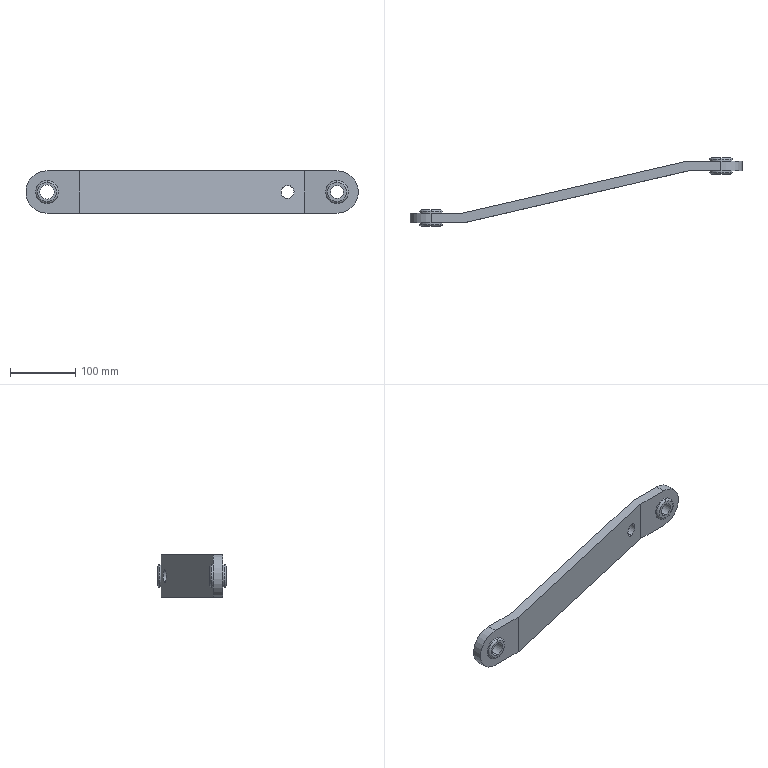Part | SolidWorks | 1 solid | 36 faces | box 510.518 x 105 x 65 mm | volume 489274 mm3 | cylinder 16 | plane 12 | torus 8 | commonest cylinder face diameters 35 x8 20 x4 22 x2 65 x2
STEP:
#1=CARTESIAN_POINT('',(396.018,97.,-17.5));
#2=VERTEX_POINT('',#1);
#3=CARTESIAN_POINT('',(396.018,97.,17.5));
#4=VERTEX_POINT('',#3);
#5=CARTESIAN_POINT('',(396.018,97.,0.));
#6=DIRECTION('',(0.,-1.,0.));
#7=DIRECTION('',(0.,0.,1.));
#8=AXIS2_PLACEMENT_3D('',#5,#6,#7);
#9=CIRCLE('',#8,17.5);
#10=EDGE_CURVE('',#2,#4,#9,.T.);
#11=ORIENTED_EDGE('',*,*,#10,.F.);
#12=CARTESIAN_POINT('',(396.018,100.,-14.5));
#13=VERTEX_POINT('',#12);
#14=CARTESIAN_POINT('',(396.018,97.,-14.5));
#15=DIRECTION('',(1.,0.,0.));
#16=DIRECTION('',(0.,0.,-1.));
#17=AXIS2_PLACEMENT_3D('',#14,#15,#16);
#18=CIRCLE('',#17,3.);
#19=EDGE_CURVE('',#2,#13,#18,.T.);
#20=ORIENTED_EDGE('',*,*,#19,.T.);
#21=CARTESIAN_POINT('',(396.018,100.,14.5));
#22=VERTEX_POINT('',#21);
#23=CARTESIAN_POINT('',(396.018,100.,0.));
#24=DIRECTION('',(0.,1.,0.));
#25=DIRECTION('',(0.,0.,1.));
#26=AXIS2_PLACEMENT_3D('',#23,#24,#25);
#27=CIRCLE('',#26,14.5);
#28=EDGE_CURVE('',#22,#13,#27,.T.);
#29=ORIENTED_EDGE('',*,*,#28,.F.);
#30=CARTESIAN_POINT('',(396.018,97.,14.5));
#31=DIRECTION('',(-1.,0.,0.));
#32=DIRECTION('',(0.,0.,1.));
#33=AXIS2_PLACEMENT_3D('',#30,#31,#32);
#34=CIRCLE('',#33,3.);
#35=EDGE_CURVE('',#4,#22,#34,.T.);
#36=ORIENTED_EDGE('',*,*,#35,.F.);
#37=EDGE_LOOP('',(#11,#20,#29,#36));
#38=FACE_OUTER_BOUND('',#37,.T.);
#39=CARTESIAN_POINT('',(396.018,97.,0.));
#40=DIRECTION('',(0.,1.,0.));
#41=DIRECTION('',(0.,0.,1.));
#42=AXIS2_PLACEMENT_3D('',#39,#40,#41);
#43=TOROIDAL_SURFACE('',#42,14.5,3.);
#44=ADVANCED_FACE('',(#38),#43,.T.);
#45=CARTESIAN_POINT('',(396.018,75.,-14.5));
#46=VERTEX_POINT('',#45);
#47=CARTESIAN_POINT('',(396.018,75.,14.5));
#48=VERTEX_POINT('',#47);
#49=CARTESIAN_POINT('',(396.018,75.,0.));
#50=DIRECTION('',(0.,-1.,0.));
#51=DIRECTION('',(0.,0.,1.));
#52=AXIS2_PLACEMENT_3D('',#49,#50,#51);
#53=CIRCLE('',#52,14.5);
#54=EDGE_CURVE('',#46,#48,#53,.T.);
#55=ORIENTED_EDGE('',*,*,#54,.F.);
#56=CARTESIAN_POINT('',(396.018,78.,-17.5));
#57=VERTEX_POINT('',#56);
#58=CARTESIAN_POINT('',(396.018,78.,-14.5));
#59=DIRECTION('',(1.,0.,0.));
#60=DIRECTION('',(0.,0.,-1.));
#61=AXIS2_PLACEMENT_3D('',#58,#59,#60);
#62=CIRCLE('',#61,3.);
#63=EDGE_CURVE('',#46,#57,#62,.T.);
#64=ORIENTED_EDGE('',*,*,#63,.T.);
#65=CARTESIAN_POINT('',(396.018,78.,17.5));
#66=VERTEX_POINT('',#65);
#67=CARTESIAN_POINT('',(396.018,78.,0.));
#68=DIRECTION('',(0.,1.,0.));
#69=DIRECTION('',(0.,0.,1.));
#70=AXIS2_PLACEMENT_3D('',#67,#68,#69);
#71=CIRCLE('',#70,17.5);
#72=EDGE_CURVE('',#66,#57,#71,.T.);
#73=ORIENTED_EDGE('',*,*,#72,.F.);
#74=CARTESIAN_POINT('',(396.018,78.,14.5));
#75=DIRECTION('',(-1.,0.,0.));
#76=DIRECTION('',(0.,0.,1.));
#77=AXIS2_PLACEMENT_3D('',#74,#75,#76);
#78=CIRCLE('',#77,3.);
#79=EDGE_CURVE('',#48,#66,#78,.T.);
#80=ORIENTED_EDGE('',*,*,#79,.F.);
#81=EDGE_LOOP('',(#55,#64,#73,#80));
#82=FACE_OUTER_BOUND('',#81,.T.);
#83=CARTESIAN_POINT('',(396.018,78.,0.));
#84=DIRECTION('',(0.,1.,0.));
#85=DIRECTION('',(0.,0.,1.));
#86=AXIS2_PLACEMENT_3D('',#83,#84,#85);
#87=TOROIDAL_SURFACE('',#86,14.5,3.);
#88=ADVANCED_FACE('',(#82),#87,.T.);
#89=ORIENTED_EDGE('',*,*,#72,.T.);
#90=CARTESIAN_POINT('',(396.018,80.,-17.5));
#91=VERTEX_POINT('',#90);
#92=CARTESIAN_POINT('',(396.018,75.,-17.5));
#93=DIRECTION('',(0.,1.,0.));
#94=VECTOR('',#93,1000.);
#95=LINE('',#92,#94);
#96=EDGE_CURVE('',#57,#91,#95,.T.);
#97=ORIENTED_EDGE('',*,*,#96,.T.);
#98=CARTESIAN_POINT('',(396.018,80.,17.5));
#99=VERTEX_POINT('',#98);
#100=CARTESIAN_POINT('',(396.018,80.,0.));
#101=DIRECTION('',(0.,-1.,0.));
#102=DIRECTION('',(0.,0.,-1.));
#103=AXIS2_PLACEMENT_3D('',#100,#101,#102);
#104=CIRCLE('',#103,17.5);
#105=EDGE_CURVE('',#91,#99,#104,.T.);
#106=ORIENTED_EDGE('',*,*,#105,.T.);
#107=CARTESIAN_POINT('',(396.018,75.,17.5));
#108=DIRECTION('',(0.,1.,0.));
#109=VECTOR('',#108,1000.);
#110=LINE('',#107,#109);
#111=EDGE_CURVE('',#66,#99,#110,.T.);
#112=ORIENTED_EDGE('',*,*,#111,.F.);
#113=EDGE_LOOP('',(#89,#97,#106,#112));
#114=FACE_OUTER_BOUND('',#113,.T.);
#115=CARTESIAN_POINT('',(396.018,75.,0.));
#116=DIRECTION('',(0.,1.,0.));
#117=DIRECTION('',(0.,0.,1.));
#118=AXIS2_PLACEMENT_3D('',#115,#116,#117);
#119=CYLINDRICAL_SURFACE('',#118,17.5);
#120=ADVANCED_FACE('',(#114),#119,.T.);
#121=CARTESIAN_POINT('',(396.018,75.,10.));
#122=VERTEX_POINT('',#121);
#123=CARTESIAN_POINT('',(396.018,75.,-10.));
#124=VERTEX_POINT('',#123);
#125=CARTESIAN_POINT('',(396.018,75.,0.));
#126=DIRECTION('',(0.,-1.,0.));
#127=DIRECTION('',(0.,0.,1.));
#128=AXIS2_PLACEMENT_3D('',#125,#126,#127);
#129=CIRCLE('',#128,10.);
#130=EDGE_CURVE('',#122,#124,#129,.T.);
#131=ORIENTED_EDGE('',*,*,#130,.T.);
#132=CARTESIAN_POINT('',(396.018,100.,-10.));
#133=VERTEX_POINT('',#132);
#134=CARTESIAN_POINT('',(396.018,-144.,-10.));
#135=DIRECTION('',(0.,1.,0.));
#136=VECTOR('',#135,1000.);
#137=LINE('',#134,#136);
#138=EDGE_CURVE('',#124,#133,#137,.T.);
#139=ORIENTED_EDGE('',*,*,#138,.T.);
#140=CARTESIAN_POINT('',(396.018,100.,10.));
#141=VERTEX_POINT('',#140);
#142=CARTESIAN_POINT('',(396.018,100.,0.));
#143=DIRECTION('',(0.,-1.,0.));
#144=DIRECTION('',(0.,0.,1.));
#145=AXIS2_PLACEMENT_3D('',#142,#143,#144);
#146=CIRCLE('',#145,10.);
#147=EDGE_CURVE('',#141,#133,#146,.T.);
#148=ORIENTED_EDGE('',*,*,#147,.F.);
#149=CARTESIAN_POINT('',(396.018,-144.,10.));
#150=DIRECTION('',(0.,1.,0.));
#151=VECTOR('',#150,1000.);
#152=LINE('',#149,#151);
#153=EDGE_CURVE('',#122,#141,#152,.T.);
#154=ORIENTED_EDGE('',*,*,#153,.F.);
#155=EDGE_LOOP('',(#131,#139,#148,#154));
#156=FACE_OUTER_BOUND('',#155,.T.);
#157=CARTESIAN_POINT('',(396.018,-144.,0.));
#158=DIRECTION('',(0.,1.,0.));
#159=DIRECTION('',(0.,0.,1.));
#160=AXIS2_PLACEMENT_3D('',#157,#158,#159);
#161=CYLINDRICAL_SURFACE('',#160,10.);
#162=ADVANCED_FACE('',(#156),#161,.F.);
#163=CARTESIAN_POINT('',(396.018,95.,-17.5));
#164=VERTEX_POINT('',#163);
#165=CARTESIAN_POINT('',(396.018,95.,17.5));
#166=VERTEX_POINT('',#165);
#167=CARTESIAN_POINT('',(396.018,95.,0.));
#168=DIRECTION('',(0.,-1.,0.));
#169=DIRECTION('',(0.,0.,-1.));
#170=AXIS2_PLACEMENT_3D('',#167,#168,#169);
#171=CIRCLE('',#170,17.5);
#172=EDGE_CURVE('',#164,#166,#171,.T.);
#173=ORIENTED_EDGE('',*,*,#172,.F.);
#174=CARTESIAN_POINT('',(396.018,75.,-17.5));
#175=DIRECTION('',(0.,1.,0.));
#176=VECTOR('',#175,1000.);
#177=LINE('',#174,#176);
#178=EDGE_CURVE('',#164,#2,#177,.T.);
#179=ORIENTED_EDGE('',*,*,#178,.T.);
#180=ORIENTED_EDGE('',*,*,#10,.T.);
#181=CARTESIAN_POINT('',(396.018,75.,17.5));
#182=DIRECTION('',(0.,1.,0.));
#183=VECTOR('',#182,1000.);
#184=LINE('',#181,#183);
#185=EDGE_CURVE('',#166,#4,#184,.T.);
#186=ORIENTED_EDGE('',*,*,#185,.F.);
#187=EDGE_LOOP('',(#173,#179,#180,#186));
#188=FACE_OUTER_BOUND('',#187,.T.);
#189=CARTESIAN_POINT('',(396.018,75.,0.));
#190=DIRECTION('',(0.,1.,0.));
#191=DIRECTION('',(0.,0.,1.));
#192=AXIS2_PLACEMENT_3D('',#189,#190,#191);
#193=CYLINDRICAL_SURFACE('',#192,17.5);
#194=ADVANCED_FACE('',(#188),#193,.T.);
#195=CARTESIAN_POINT('',(-49.5,17.,-17.5));
#196=VERTEX_POINT('',#195);
#197=CARTESIAN_POINT('',(-49.5,17.,17.5));
#198=VERTEX_POINT('',#197);
#199=CARTESIAN_POINT('',(-49.5,17.,0.));
#200=DIRECTION('',(0.,-1.,0.));
#201=DIRECTION('',(0.,0.,1.));
#202=AXIS2_PLACEMENT_3D('',#199,#200,#201);
#203=CIRCLE('',#202,17.5);
#204=EDGE_CURVE('',#196,#198,#203,.T.);
#205=ORIENTED_EDGE('',*,*,#204,.F.);
#206=CARTESIAN_POINT('',(-49.5,20.,-14.5));
#207=VERTEX_POINT('',#206);
#208=CARTESIAN_POINT('',(-49.5,17.,-14.5));
#209=DIRECTION('',(1.,0.,0.));
#210=DIRECTION('',(0.,0.,-1.));
#211=AXIS2_PLACEMENT_3D('',#208,#209,#210);
#212=CIRCLE('',#211,3.);
#213=EDGE_CURVE('',#196,#207,#212,.T.);
#214=ORIENTED_EDGE('',*,*,#213,.T.);
#215=CARTESIAN_POINT('',(-49.5,20.,14.5));
#216=VERTEX_POINT('',#215);
#217=CARTESIAN_POINT('',(-49.5,20.,0.));
#218=DIRECTION('',(0.,1.,0.));
#219=DIRECTION('',(0.,0.,1.));
#220=AXIS2_PLACEMENT_3D('',#217,#218,#219);
#221=CIRCLE('',#220,14.5);
#222=EDGE_CURVE('',#216,#207,#221,.T.);
#223=ORIENTED_EDGE('',*,*,#222,.F.);
#224=CARTESIAN_POINT('',(-49.5,17.,14.5));
#225=DIRECTION('',(-1.,0.,0.));
#226=DIRECTION('',(0.,0.,1.));
#227=AXIS2_PLACEMENT_3D('',#224,#225,#226);
#228=CIRCLE('',#227,3.);
#229=EDGE_CURVE('',#198,#216,#228,.T.);
#230=ORIENTED_EDGE('',*,*,#229,.F.);
#231=EDGE_LOOP('',(#205,#214,#223,#230));
#232=FACE_OUTER_BOUND('',#231,.T.);
#233=CARTESIAN_POINT('',(-49.5,17.,0.));
#234=DIRECTION('',(0.,1.,0.));
#235=DIRECTION('',(0.,0.,1.));
#236=AXIS2_PLACEMENT_3D('',#233,#234,#235);
#237=TOROIDAL_SURFACE('',#236,14.5,3.);
#238=ADVANCED_FACE('',(#232),#237,.T.);
#239=CARTESIAN_POINT('',(-49.5,-5.,-14.5));
#240=VERTEX_POINT('',#239);
#241=CARTESIAN_POINT('',(-49.5,-5.,14.5));
#242=VERTEX_POINT('',#241);
#243=CARTESIAN_POINT('',(-49.5,-5.,0.));
#244=DIRECTION('',(0.,-1.,0.));
#245=DIRECTION('',(0.,0.,1.));
#246=AXIS2_PLACEMENT_3D('',#243,#244,#245);
#247=CIRCLE('',#246,14.5);
#248=EDGE_CURVE('',#240,#242,#247,.T.);
#249=ORIENTED_EDGE('',*,*,#248,.F.);
#250=CARTESIAN_POINT('',(-49.5,-2.,-17.5));
#251=VERTEX_POINT('',#250);
#252=CARTESIAN_POINT('',(-49.5,-2.,-14.5));
#253=DIRECTION('',(1.,0.,0.));
#254=DIRECTION('',(0.,0.,-1.));
#255=AXIS2_PLACEMENT_3D('',#252,#253,#254);
#256=CIRCLE('',#255,3.);
#257=EDGE_CURVE('',#240,#251,#256,.T.);
#258=ORIENTED_EDGE('',*,*,#257,.T.);
#259=CARTESIAN_POINT('',(-49.5,-2.,17.5));
#260=VERTEX_POINT('',#259);
#261=CARTESIAN_POINT('',(-49.5,-2.,0.));
#262=DIRECTION('',(0.,1.,0.));
#263=DIRECTION('',(0.,0.,1.));
#264=AXIS2_PLACEMENT_3D('',#261,#262,#263);
#265=CIRCLE('',#264,17.5);
#266=EDGE_CURVE('',#260,#251,#265,.T.);
#267=ORIENTED_EDGE('',*,*,#266,.F.);
#268=CARTESIAN_POINT('',(-49.5,-2.,14.5));
#269=DIRECTION('',(-1.,0.,0.));
#270=DIRECTION('',(0.,0.,1.));
#271=AXIS2_PLACEMENT_3D('',#268,#269,#270);
#272=CIRCLE('',#271,3.);
#273=EDGE_CURVE('',#242,#260,#272,.T.);
#274=ORIENTED_EDGE('',*,*,#273,.F.);
#275=EDGE_LOOP('',(#249,#258,#267,#274));
#276=FACE_OUTER_BOUND('',#275,.T.);
#277=CARTESIAN_POINT('',(-49.5,-2.,0.));
#278=DIRECTION('',(0.,1.,0.));
#279=DIRECTION('',(0.,0.,1.));
#280=AXIS2_PLACEMENT_3D('',#277,#278,#279);
#281=TOROIDAL_SURFACE('',#280,14.5,3.);
#282=ADVANCED_FACE('',(#276),#281,.T.);
#283=ORIENTED_EDGE('',*,*,#266,.T.);
#284=CARTESIAN_POINT('',(-49.5,0.,-17.5));
#285=VERTEX_POINT('',#284);
#286=CARTESIAN_POINT('',(-49.5,-5.,-17.5));
#287=DIRECTION('',(0.,1.,0.));
#288=VECTOR('',#287,1000.);
#289=LINE('',#286,#288);
#290=EDGE_CURVE('',#251,#285,#289,.T.);
#291=ORIENTED_EDGE('',*,*,#290,.T.);
#292=CARTESIAN_POINT('',(-49.5,0.,17.5));
#293=VERTEX_POINT('',#292);
#294=CARTESIAN_POINT('',(-49.5,0.,0.));
#295=DIRECTION('',(0.,-1.,0.));
#296=DIRECTION('',(0.,0.,-1.));
#297=AXIS2_PLACEMENT_3D('',#294,#295,#296);
#298=CIRCLE('',#297,17.5);
#299=EDGE_CURVE('',#285,#293,#298,.T.);
#300=ORIENTED_EDGE('',*,*,#299,.T.);
#301=CARTESIAN_POINT('',(-49.5,-5.,17.5));
#302=DIRECTION('',(0.,1.,0.));
#303=VECTOR('',#302,1000.);
#304=LINE('',#301,#303);
#305=EDGE_CURVE('',#260,#293,#304,.T.);
#306=ORIENTED_EDGE('',*,*,#305,.F.);
#307=EDGE_LOOP('',(#283,#291,#300,#306));
#308=FACE_OUTER_BOUND('',#307,.T.);
#309=CARTESIAN_POINT('',(-49.5,-5.,0.));
#310=DIRECTION('',(0.,1.,0.));
#311=DIRECTION('',(0.,0.,1.));
#312=AXIS2_PLACEMENT_3D('',#309,#310,#311);
#313=CYLINDRICAL_SURFACE('',#312,17.5);
#314=ADVANCED_FACE('',(#308),#313,.T.);
#315=CARTESIAN_POINT('',(-49.5,-5.,11.));
#316=VERTEX_POINT('',#315);
#317=CARTESIAN_POINT('',(-49.5,-5.,-11.));
#318=VERTEX_POINT('',#317);
#319=CARTESIAN_POINT('',(-49.5,-5.,0.));
#320=DIRECTION('',(0.,-1.,0.));
#321=DIRECTION('',(0.,0.,1.));
#322=AXIS2_PLACEMENT_3D('',#319,#320,#321);
#323=CIRCLE('',#322,11.);
#324=EDGE_CURVE('',#316,#318,#323,.T.);
#325=ORIENTED_EDGE('',*,*,#324,.T.);
#326=CARTESIAN_POINT('',(-49.5,20.,-11.));
#327=VERTEX_POINT('',#326);
#328=CARTESIAN_POINT('',(-49.5,-144.,-11.));
#329=DIRECTION('',(0.,1.,0.));
#330=VECTOR('',#329,1000.);
#331=LINE('',#328,#330);
#332=EDGE_CURVE('',#318,#327,#331,.T.);
#333=ORIENTED_EDGE('',*,*,#332,.T.);
#334=CARTESIAN_POINT('',(-49.5,20.,11.));
#335=VERTEX_POINT('',#334);
#336=CARTESIAN_POINT('',(-49.5,20.,0.));
#337=DIRECTION('',(0.,-1.,0.));
#338=DIRECTION('',(0.,0.,1.));
#339=AXIS2_PLACEMENT_3D('',#336,#337,#338);
#340=CIRCLE('',#339,11.);
#341=EDGE_CURVE('',#335,#327,#340,.T.);
#342=ORIENTED_EDGE('',*,*,#341,.F.);
#343=CARTESIAN_POINT('',(-49.5,-144.,11.));
#344=DIRECTION('',(0.,1.,0.));
#345=VECTOR('',#344,1000.);
#346=LINE('',#343,#345);
#347=EDGE_CURVE('',#316,#335,#346,.T.);
#348=ORIENTED_EDGE('',*,*,#347,.F.);
#349=EDGE_LOOP('',(#325,#333,#342,#348));
#350=FACE_OUTER_BOUND('',#349,.T.);
#351=CARTESIAN_POINT('',(-49.5,-144.,0.));
#352=DIRECTION('',(0.,1.,0.));
#353=DIRECTION('',(0.,0.,1.));
#354=AXIS2_PLACEMENT_3D('',#351,#352,#353);
#355=CYLINDRICAL_SURFACE('',#354,11.);
#356=ADVANCED_FACE('',(#350),#355,.F.);
#357=CARTESIAN_POINT('',(-49.5,15.,-17.5));
#358=VERTEX_POINT('',#357);
#359=CARTESIAN_POINT('',(-49.5,15.,17.5));
#360=VERTEX_POINT('',#359);
#361=CARTESIAN_POINT('',(-49.5,15.,0.));
#362=DIRECTION('',(0.,-1.,0.));
#363=DIRECTION('',(0.,0.,-1.));
#364=AXIS2_PLACEMENT_3D('',#361,#362,#363);
#365=CIRCLE('',#364,17.5);
#366=EDGE_CURVE('',#358,#360,#365,.T.);
#367=ORIENTED_EDGE('',*,*,#366,.F.);
#368=CARTESIAN_POINT('',(-49.5,-5.,-17.5));
#369=DIRECTION('',(0.,1.,0.));
#370=VECTOR('',#369,1000.);
#371=LINE('',#368,#370);
#372=EDGE_CURVE('',#358,#196,#371,.T.);
#373=ORIENTED_EDGE('',*,*,#372,.T.);
#374=ORIENTED_EDGE('',*,*,#204,.T.);
#375=CARTESIAN_POINT('',(-49.5,-5.,17.5));
#376=DIRECTION('',(0.,1.,0.));
#377=VECTOR('',#376,1000.);
#378=LINE('',#375,#377);
#379=EDGE_CURVE('',#360,#198,#378,.T.);
#380=ORIENTED_EDGE('',*,*,#379,.F.);
#381=EDGE_LOOP('',(#367,#373,#374,#380));
#382=FACE_OUTER_BOUND('',#381,.T.);
#383=CARTESIAN_POINT('',(-49.5,-5.,0.));
#384=DIRECTION('',(0.,1.,0.));
#385=DIRECTION('',(0.,0.,1.));
#386=AXIS2_PLACEMENT_3D('',#383,#384,#385);
#387=CYLINDRICAL_SURFACE('',#386,17.5);
#388=ADVANCED_FACE('',(#382),#387,.T.);
#389=CARTESIAN_POINT('',(320.,73.878,10.));
#390=VERTEX_POINT('',#389);
#391=CARTESIAN_POINT('',(320.,73.878,-10.));
#392=VERTEX_POINT('',#391);
#393=CARTESIAN_POINT('',(320.,73.878,10.));
#394=CARTESIAN_POINT('',(300.,69.26,10.));
#395=CARTESIAN_POINT('',(300.,69.26,-10.));
#396=CARTESIAN_POINT('',(320.,73.878,-10.));
#397=(BOUNDED_CURVE()B_SPLINE_CURVE(3,(#393,#394,#395,#396),.UNSPECIFIED.,.F.,.F.)B_SPLINE_CURVE_WITH_KNOTS((4,4),(1.571,4.712),.UNSPECIFIED.)CURVE()GEOMETRIC_REPRESENTATION_ITEM()RATIONAL_B_SPLINE_CURVE((1.,0.3333,0.3333,1.))REPRESENTATION_ITEM(''));
#398=EDGE_CURVE('',#390,#392,#397,.T.);
#399=ORIENTED_EDGE('',*,*,#398,.T.);
#400=CARTESIAN_POINT('',(320.,89.272,-10.));
#401=VERTEX_POINT('',#400);
#402=CARTESIAN_POINT('',(320.,-144.,-10.));
#403=DIRECTION('',(0.,1.,0.));
#404=VECTOR('',#403,1000.);
#405=LINE('',#402,#404);
#406=EDGE_CURVE('',#392,#401,#405,.T.);
#407=ORIENTED_EDGE('',*,*,#406,.T.);
#408=CARTESIAN_POINT('',(320.,89.272,10.));
#409=VERTEX_POINT('',#408);
#410=CARTESIAN_POINT('',(320.,89.272,10.));
#411=CARTESIAN_POINT('',(300.,84.655,10.));
#412=CARTESIAN_POINT('',(300.,84.655,-10.));
#413=CARTESIAN_POINT('',(320.,89.272,-10.));
#414=(BOUNDED_CURVE()B_SPLINE_CURVE(3,(#410,#411,#412,#413),.UNSPECIFIED.,.F.,.F.)B_SPLINE_CURVE_WITH_KNOTS((4,4),(1.571,4.712),.UNSPECIFIED.)CURVE()GEOMETRIC_REPRESENTATION_ITEM()RATIONAL_B_SPLINE_CURVE((1.,0.3333,0.3333,1.))REPRESENTATION_ITEM(''));
#415=EDGE_CURVE('',#409,#401,#414,.T.);
#416=ORIENTED_EDGE('',*,*,#415,.F.);
#417=CARTESIAN_POINT('',(320.,-144.,10.));
#418=DIRECTION('',(0.,1.,0.));
#419=VECTOR('',#418,1000.);
#420=LINE('',#417,#419);
#421=EDGE_CURVE('',#390,#409,#420,.T.);
#422=ORIENTED_EDGE('',*,*,#421,.F.);
#423=EDGE_LOOP('',(#399,#407,#416,#422));
#424=FACE_OUTER_BOUND('',#423,.T.);
#425=CARTESIAN_POINT('',(320.,-144.,0.));
#426=DIRECTION('',(0.,1.,0.));
#427=DIRECTION('',(0.,0.,1.));
#428=AXIS2_PLACEMENT_3D('',#425,#426,#427);
#429=CYLINDRICAL_SURFACE('',#428,10.);
#430=ADVANCED_FACE('',(#424),#429,.F.);
#431=CARTESIAN_POINT('',(396.018,95.,-32.5));
#432=VERTEX_POINT('',#431);
#433=CARTESIAN_POINT('',(396.018,80.,-32.5));
#434=VERTEX_POINT('',#433);
#435=CARTESIAN_POINT('',(396.018,80.,-32.5));
#436=DIRECTION('',(0.,-1.,0.));
#437=VECTOR('',#436,1000.);
#438=LINE('',#435,#437);
#439=EDGE_CURVE('',#432,#434,#438,.T.);
#440=ORIENTED_EDGE('',*,*,#439,.F.);
#441=CARTESIAN_POINT('',(396.018,95.,32.5));
#442=VERTEX_POINT('',#441);
#443=CARTESIAN_POINT('',(396.018,95.,0.));
#444=DIRECTION('',(0.,1.,0.));
#445=DIRECTION('',(0.,0.,-1.));
#446=AXIS2_PLACEMENT_3D('',#443,#444,#445);
#447=CIRCLE('',#446,32.5);
#448=EDGE_CURVE('',#442,#432,#447,.T.);
#449=ORIENTED_EDGE('',*,*,#448,.F.);
#450=CARTESIAN_POINT('',(396.018,80.,32.5));
#451=VERTEX_POINT('',#450);
#452=CARTESIAN_POINT('',(396.018,0.,32.5));
#453=DIRECTION('',(0.,1.,0.));
#454=VECTOR('',#453,1000.);
#455=LINE('',#452,#454);
#456=EDGE_CURVE('',#451,#442,#455,.T.);
#457=ORIENTED_EDGE('',*,*,#456,.F.);
#458=CARTESIAN_POINT('',(396.018,80.,0.));
#459=DIRECTION('',(0.,-1.,0.));
#460=DIRECTION('',(0.,0.,-1.));
#461=AXIS2_PLACEMENT_3D('',#458,#459,#460);
#462=CIRCLE('',#461,32.5);
#463=EDGE_CURVE('',#434,#451,#462,.T.);
#464=ORIENTED_EDGE('',*,*,#463,.F.);
#465=EDGE_LOOP('',(#440,#449,#457,#464));
#466=FACE_OUTER_BOUND('',#465,.T.);
#467=CARTESIAN_POINT('',(396.018,95.,0.));
#468=DIRECTION('',(0.,-1.,0.));
#469=DIRECTION('',(0.,0.,-1.));
#470=AXIS2_PLACEMENT_3D('',#467,#468,#469);
#471=CYLINDRICAL_SURFACE('',#470,32.5);
#472=ADVANCED_FACE('',(#466),#471,.T.);
#473=CARTESIAN_POINT('',(-49.5,15.,32.5));
#474=VERTEX_POINT('',#473);
#475=CARTESIAN_POINT('',(-49.5,0.,32.5));
#476=VERTEX_POINT('',#475);
#477=CARTESIAN_POINT('',(-49.5,0.,32.5));
#478=DIRECTION('',(0.,-1.,0.));
#479=VECTOR('',#478,1000.);
#480=LINE('',#477,#479);
#481=EDGE_CURVE('',#474,#476,#480,.T.);
#482=ORIENTED_EDGE('',*,*,#481,.F.);
#483=CARTESIAN_POINT('',(-49.5,15.,-32.5));
#484=VERTEX_POINT('',#483);
#485=CARTESIAN_POINT('',(-49.5,15.,0.));
#486=DIRECTION('',(0.,1.,0.));
#487=DIRECTION('',(0.,0.,-1.));
#488=AXIS2_PLACEMENT_3D('',#485,#486,#487);
#489=CIRCLE('',#488,32.5);
#490=EDGE_CURVE('',#484,#474,#489,.T.);
#491=ORIENTED_EDGE('',*,*,#490,.F.);
#492=CARTESIAN_POINT('',(-49.5,0.,-32.5));
#493=VERTEX_POINT('',#492);
#494=CARTESIAN_POINT('',(-49.5,80.,-32.5));
#495=DIRECTION('',(0.,1.,0.));
#496=VECTOR('',#495,1000.);
#497=LINE('',#494,#496);
#498=EDGE_CURVE('',#493,#484,#497,.T.);
#499=ORIENTED_EDGE('',*,*,#498,.F.);
#500=CARTESIAN_POINT('',(-49.5,0.,0.));
#501=DIRECTION('',(0.,-1.,0.));
#502=DIRECTION('',(0.,0.,-1.));
#503=AXIS2_PLACEMENT_3D('',#500,#501,#502);
#504=CIRCLE('',#503,32.5);
#505=EDGE_CURVE('',#476,#493,#504,.T.);
#506=ORIENTED_EDGE('',*,*,#505,.F.);
#507=EDGE_LOOP('',(#482,#491,#499,#506));
#508=FACE_OUTER_BOUND('',#507,.T.);
#509=CARTESIAN_POINT('',(-49.5,15.,0.));
#510=DIRECTION('',(0.,-1.,0.));
#511=DIRECTION('',(0.,0.,-1.));
#512=AXIS2_PLACEMENT_3D('',#509,#510,#511);
#513=CYLINDRICAL_SURFACE('',#512,32.5);
#514=ADVANCED_FACE('',(#508),#513,.T.);
#515=CARTESIAN_POINT('',(344.809,95.,-32.5));
#516=VERTEX_POINT('',#515);
#517=CARTESIAN_POINT('',(346.518,95.,-32.5));
#518=DIRECTION('',(1.,0.,0.));
#519=VECTOR('',#518,1000.);
#520=LINE('',#517,#519);
#521=EDGE_CURVE('',#516,#432,#520,.T.);
#522=ORIENTED_EDGE('',*,*,#521,.T.);
#523=ORIENTED_EDGE('',*,*,#439,.T.);
#524=CARTESIAN_POINT('',(346.518,80.,-32.5));
#525=VERTEX_POINT('',#524);
#526=CARTESIAN_POINT('',(346.518,80.,-32.5));
#527=DIRECTION('',(1.,0.,0.));
#528=VECTOR('',#527,1000.);
#529=LINE('',#526,#528);
#530=EDGE_CURVE('',#525,#434,#529,.T.);
#531=ORIENTED_EDGE('',*,*,#530,.F.);
#532=CARTESIAN_POINT('',(0.,0.,-32.5));
#533=VERTEX_POINT('',#532);
#534=CARTESIAN_POINT('',(0.,0.,-32.5));
#535=DIRECTION('',(0.9744,0.225,0.));
#536=VECTOR('',#535,1000.);
#537=LINE('',#534,#536);
#538=EDGE_CURVE('',#533,#525,#537,.T.);
#539=ORIENTED_EDGE('',*,*,#538,.F.);
#540=CARTESIAN_POINT('',(-82.,0.,-32.5));
#541=DIRECTION('',(1.,0.,0.));
#542=VECTOR('',#541,1000.);
#543=LINE('',#540,#542);
#544=EDGE_CURVE('',#493,#533,#543,.T.);
#545=ORIENTED_EDGE('',*,*,#544,.F.);
#546=ORIENTED_EDGE('',*,*,#498,.T.);
#547=CARTESIAN_POINT('',(-1.709,15.,-32.5));
#548=VERTEX_POINT('',#547);
#549=CARTESIAN_POINT('',(-82.,15.,-32.5));
#550=DIRECTION('',(1.,0.,0.));
#551=VECTOR('',#550,1000.);
#552=LINE('',#549,#551);
#553=EDGE_CURVE('',#484,#548,#552,.T.);
#554=ORIENTED_EDGE('',*,*,#553,.T.);
#555=CARTESIAN_POINT('',(-3.374,14.616,-32.5));
#556=DIRECTION('',(0.9744,0.225,0.));
#557=VECTOR('',#556,1000.);
#558=LINE('',#555,#557);
#559=EDGE_CURVE('',#548,#516,#558,.T.);
#560=ORIENTED_EDGE('',*,*,#559,.T.);
#561=EDGE_LOOP('',(#522,#523,#531,#539,#545,#546,#554,#560));
#562=FACE_OUTER_BOUND('',#561,.T.);
#563=CARTESIAN_POINT('',(346.518,80.,-32.5));
#564=DIRECTION('',(0.,0.,-1.));
#565=DIRECTION('',(1.,0.,0.));
#566=AXIS2_PLACEMENT_3D('',#563,#564,#565);
#567=PLANE('',#566);
#568=ADVANCED_FACE('',(#562),#567,.T.);
#569=CARTESIAN_POINT('',(346.518,80.,32.5));
#570=VERTEX_POINT('',#569);
#571=CARTESIAN_POINT('',(346.518,80.,32.5));
#572=DIRECTION('',(1.,0.,0.));
#573=VECTOR('',#572,1000.);
#574=LINE('',#571,#573);
#575=EDGE_CURVE('',#570,#451,#574,.T.);
#576=ORIENTED_EDGE('',*,*,#575,.T.);
#577=ORIENTED_EDGE('',*,*,#456,.T.);
#578=CARTESIAN_POINT('',(344.809,95.,32.5));
#579=VERTEX_POINT('',#578);
#580=CARTESIAN_POINT('',(346.518,95.,32.5));
#581=DIRECTION('',(1.,0.,0.));
#582=VECTOR('',#581,1000.);
#583=LINE('',#580,#582);
#584=EDGE_CURVE('',#579,#442,#583,.T.);
#585=ORIENTED_EDGE('',*,*,#584,.F.);
#586=CARTESIAN_POINT('',(-1.709,15.,32.5));
#587=VERTEX_POINT('',#586);
#588=CARTESIAN_POINT('',(-3.374,14.616,32.5));
#589=DIRECTION('',(0.9744,0.225,0.));
#590=VECTOR('',#589,1000.);
#591=LINE('',#588,#590);
#592=EDGE_CURVE('',#587,#579,#591,.T.);
#593=ORIENTED_EDGE('',*,*,#592,.F.);
#594=CARTESIAN_POINT('',(-82.,15.,32.5));
#595=DIRECTION('',(1.,0.,0.));
#596=VECTOR('',#595,1000.);
#597=LINE('',#594,#596);
#598=EDGE_CURVE('',#474,#587,#597,.T.);
#599=ORIENTED_EDGE('',*,*,#598,.F.);
#600=ORIENTED_EDGE('',*,*,#481,.T.);
#601=CARTESIAN_POINT('',(0.,0.,32.5));
#602=VERTEX_POINT('',#601);
#603=CARTESIAN_POINT('',(-82.,0.,32.5));
#604=DIRECTION('',(1.,0.,0.));
#605=VECTOR('',#604,1000.);
#606=LINE('',#603,#605);
#607=EDGE_CURVE('',#476,#602,#606,.T.);
#608=ORIENTED_EDGE('',*,*,#607,.T.);
#609=CARTESIAN_POINT('',(0.,0.,32.5));
#610=DIRECTION('',(0.9744,0.225,0.));
#611=VECTOR('',#610,1000.);
#612=LINE('',#609,#611);
#613=EDGE_CURVE('',#602,#570,#612,.T.);
#614=ORIENTED_EDGE('',*,*,#613,.T.);
#615=EDGE_LOOP('',(#576,#577,#585,#593,#599,#600,#608,#614));
#616=FACE_OUTER_BOUND('',#615,.T.);
#617=CARTESIAN_POINT('',(-82.,0.,32.5));
#618=DIRECTION('',(0.,0.,-1.));
#619=DIRECTION('',(1.,0.,0.));
#620=AXIS2_PLACEMENT_3D('',#617,#618,#619);
#621=PLANE('',#620);
#622=ADVANCED_FACE('',(#616),#621,.F.);
#623=CARTESIAN_POINT('',(-49.5,0.,0.));
#624=DIRECTION('',(0.,-1.,0.));
#625=DIRECTION('',(0.,0.,-1.));
#626=AXIS2_PLACEMENT_3D('',#623,#624,#625);
#627=CIRCLE('',#626,17.5);
#628=EDGE_CURVE('',#293,#285,#627,.T.);
#629=ORIENTED_EDGE('',*,*,#628,.F.);
#630=ORIENTED_EDGE('',*,*,#299,.F.);
#631=EDGE_LOOP('',(#629,#630));
#632=FACE_BOUND('',#631,.T.);
#633=ORIENTED_EDGE('',*,*,#607,.F.);
#634=ORIENTED_EDGE('',*,*,#505,.T.);
#635=ORIENTED_EDGE('',*,*,#544,.T.);
#636=CARTESIAN_POINT('',(0.,0.,-32.5));
#637=DIRECTION('',(0.,0.,1.));
#638=VECTOR('',#637,1000.);
#639=LINE('',#636,#638);
#640=EDGE_CURVE('',#533,#602,#639,.T.);
#641=ORIENTED_EDGE('',*,*,#640,.T.);
#642=EDGE_LOOP('',(#633,#634,#635,#641));
#643=FACE_OUTER_BOUND('',#642,.T.);
#644=CARTESIAN_POINT('',(-82.,0.,-32.5));
#645=DIRECTION('',(0.,-1.,0.));
#646=DIRECTION('',(0.,0.,-1.));
#647=AXIS2_PLACEMENT_3D('',#644,#645,#646);
#648=PLANE('',#647);
#649=ADVANCED_FACE('',(#632,#643),#648,.T.);
#650=ORIENTED_EDGE('',*,*,#398,.F.);
#651=CARTESIAN_POINT('',(320.,73.878,-10.));
#652=CARTESIAN_POINT('',(340.,78.495,-10.));
#653=CARTESIAN_POINT('',(340.,78.495,10.));
#654=CARTESIAN_POINT('',(320.,73.878,10.));
#655=(BOUNDED_CURVE()B_SPLINE_CURVE(3,(#651,#652,#653,#654),.UNSPECIFIED.,.F.,.F.)B_SPLINE_CURVE_WITH_KNOTS((4,4),(4.712,7.854),.UNSPECIFIED.)CURVE()GEOMETRIC_REPRESENTATION_ITEM()RATIONAL_B_SPLINE_CURVE((1.,0.3333,0.3333,1.))REPRESENTATION_ITEM(''));
#656=EDGE_CURVE('',#392,#390,#655,.T.);
#657=ORIENTED_EDGE('',*,*,#656,.F.);
#658=EDGE_LOOP('',(#650,#657));
#659=FACE_BOUND('',#658,.T.);
#660=ORIENTED_EDGE('',*,*,#613,.F.);
#661=ORIENTED_EDGE('',*,*,#640,.F.);
#662=ORIENTED_EDGE('',*,*,#538,.T.);
#663=CARTESIAN_POINT('',(346.518,80.,-32.5));
#664=DIRECTION('',(0.,0.,1.));
#665=VECTOR('',#664,1000.);
#666=LINE('',#663,#665);
#667=EDGE_CURVE('',#525,#570,#666,.T.);
#668=ORIENTED_EDGE('',*,*,#667,.T.);
#669=EDGE_LOOP('',(#660,#661,#662,#668));
#670=FACE_OUTER_BOUND('',#669,.T.);
#671=CARTESIAN_POINT('',(0.,0.,-32.5));
#672=DIRECTION('',(0.225,-0.9744,0.));
#673=DIRECTION('',(0.9744,0.225,0.));
#674=AXIS2_PLACEMENT_3D('',#671,#672,#673);
#675=PLANE('',#674);
#676=ADVANCED_FACE('',(#659,#670),#675,.T.);
#677=CARTESIAN_POINT('',(396.018,80.,0.));
#678=DIRECTION('',(0.,-1.,0.));
#679=DIRECTION('',(0.,0.,-1.));
#680=AXIS2_PLACEMENT_3D('',#677,#678,#679);
#681=CIRCLE('',#680,17.5);
#682=EDGE_CURVE('',#99,#91,#681,.T.);
#683=ORIENTED_EDGE('',*,*,#682,.F.);
#684=ORIENTED_EDGE('',*,*,#105,.F.);
#685=EDGE_LOOP('',(#683,#684));
#686=FACE_BOUND('',#685,.T.);
#687=ORIENTED_EDGE('',*,*,#530,.T.);
#688=ORIENTED_EDGE('',*,*,#463,.T.);
#689=ORIENTED_EDGE('',*,*,#575,.F.);
#690=ORIENTED_EDGE('',*,*,#667,.F.);
#691=EDGE_LOOP('',(#687,#688,#689,#690));
#692=FACE_OUTER_BOUND('',#691,.T.);
#693=CARTESIAN_POINT('',(346.518,80.,-32.5));
#694=DIRECTION('',(0.,-1.,0.));
#695=DIRECTION('',(0.,0.,-1.));
#696=AXIS2_PLACEMENT_3D('',#693,#694,#695);
#697=PLANE('',#696);
#698=ADVANCED_FACE('',(#686,#692),#697,.T.);
#699=CARTESIAN_POINT('',(-49.5,15.,0.));
#700=DIRECTION('',(0.,-1.,0.));
#701=DIRECTION('',(0.,0.,-1.));
#702=AXIS2_PLACEMENT_3D('',#699,#700,#701);
#703=CIRCLE('',#702,17.5);
#704=EDGE_CURVE('',#360,#358,#703,.T.);
#705=ORIENTED_EDGE('',*,*,#704,.T.);
#706=ORIENTED_EDGE('',*,*,#366,.T.);
#707=EDGE_LOOP('',(#705,#706));
#708=FACE_BOUND('',#707,.T.);
#709=ORIENTED_EDGE('',*,*,#553,.F.);
#710=ORIENTED_EDGE('',*,*,#490,.T.);
#711=ORIENTED_EDGE('',*,*,#598,.T.);
#712=CARTESIAN_POINT('',(-1.709,15.,-32.5));
#713=DIRECTION('',(0.,0.,1.));
#714=VECTOR('',#713,1000.);
#715=LINE('',#712,#714);
#716=EDGE_CURVE('',#548,#587,#715,.T.);
#717=ORIENTED_EDGE('',*,*,#716,.F.);
#718=EDGE_LOOP('',(#709,#710,#711,#717));
#719=FACE_OUTER_BOUND('',#718,.T.);
#720=CARTESIAN_POINT('',(-82.,15.,-32.5));
#721=DIRECTION('',(0.,-1.,0.));
#722=DIRECTION('',(0.,0.,-1.));
#723=AXIS2_PLACEMENT_3D('',#720,#721,#722);
#724=PLANE('',#723);
#725=ADVANCED_FACE('',(#708,#719),#724,.F.);
#726=ORIENTED_EDGE('',*,*,#415,.T.);
#727=CARTESIAN_POINT('',(320.,89.272,-10.));
#728=CARTESIAN_POINT('',(340.,93.89,-10.));
#729=CARTESIAN_POINT('',(340.,93.89,10.));
#730=CARTESIAN_POINT('',(320.,89.272,10.));
#731=(BOUNDED_CURVE()B_SPLINE_CURVE(3,(#727,#728,#729,#730),.UNSPECIFIED.,.F.,.F.)B_SPLINE_CURVE_WITH_KNOTS((4,4),(4.712,7.854),.UNSPECIFIED.)CURVE()GEOMETRIC_REPRESENTATION_ITEM()RATIONAL_B_SPLINE_CURVE((1.,0.3333,0.3333,1.))REPRESENTATION_ITEM(''));
#732=EDGE_CURVE('',#401,#409,#731,.T.);
#733=ORIENTED_EDGE('',*,*,#732,.T.);
#734=EDGE_LOOP('',(#726,#733));
#735=FACE_BOUND('',#734,.T.);
#736=ORIENTED_EDGE('',*,*,#592,.T.);
#737=CARTESIAN_POINT('',(344.809,95.,-32.5));
#738=DIRECTION('',(0.,0.,1.));
#739=VECTOR('',#738,1000.);
#740=LINE('',#737,#739);
#741=EDGE_CURVE('',#516,#579,#740,.T.);
#742=ORIENTED_EDGE('',*,*,#741,.F.);
#743=ORIENTED_EDGE('',*,*,#559,.F.);
#744=ORIENTED_EDGE('',*,*,#716,.T.);
#745=EDGE_LOOP('',(#736,#742,#743,#744));
#746=FACE_OUTER_BOUND('',#745,.T.);
#747=CARTESIAN_POINT('',(-3.374,14.616,-32.5));
#748=DIRECTION('',(0.225,-0.9744,0.));
#749=DIRECTION('',(0.9744,0.225,0.));
#750=AXIS2_PLACEMENT_3D('',#747,#748,#749);
#751=PLANE('',#750);
#752=ADVANCED_FACE('',(#735,#746),#751,.F.);
#753=CARTESIAN_POINT('',(396.018,95.,0.));
#754=DIRECTION('',(0.,-1.,0.));
#755=DIRECTION('',(0.,0.,-1.));
#756=AXIS2_PLACEMENT_3D('',#753,#754,#755);
#757=CIRCLE('',#756,17.5);
#758=EDGE_CURVE('',#166,#164,#757,.T.);
#759=ORIENTED_EDGE('',*,*,#758,.T.);
#760=ORIENTED_EDGE('',*,*,#172,.T.);
#761=EDGE_LOOP('',(#759,#760));
#762=FACE_BOUND('',#761,.T.);
#763=ORIENTED_EDGE('',*,*,#584,.T.);
#764=ORIENTED_EDGE('',*,*,#448,.T.);
#765=ORIENTED_EDGE('',*,*,#521,.F.);
#766=ORIENTED_EDGE('',*,*,#741,.T.);
#767=EDGE_LOOP('',(#763,#764,#765,#766));
#768=FACE_OUTER_BOUND('',#767,.T.);
#769=CARTESIAN_POINT('',(346.518,95.,-32.5));
#770=DIRECTION('',(0.,-1.,0.));
#771=DIRECTION('',(0.,0.,-1.));
#772=AXIS2_PLACEMENT_3D('',#769,#770,#771);
#773=PLANE('',#772);
#774=ADVANCED_FACE('',(#762,#768),#773,.F.);
#775=ORIENTED_EDGE('',*,*,#406,.F.);
#776=ORIENTED_EDGE('',*,*,#656,.T.);
#777=ORIENTED_EDGE('',*,*,#421,.T.);
#778=ORIENTED_EDGE('',*,*,#732,.F.);
#779=EDGE_LOOP('',(#775,#776,#777,#778));
#780=FACE_OUTER_BOUND('',#779,.T.);
#781=CARTESIAN_POINT('',(320.,-144.,0.));
#782=DIRECTION('',(0.,1.,0.));
#783=DIRECTION('',(0.,0.,1.));
#784=AXIS2_PLACEMENT_3D('',#781,#782,#783);
#785=CYLINDRICAL_SURFACE('',#784,10.);
#786=ADVANCED_FACE('',(#780),#785,.F.);
#787=ORIENTED_EDGE('',*,*,#222,.T.);
#788=CARTESIAN_POINT('',(-49.5,20.,0.));
#789=DIRECTION('',(0.,1.,0.));
#790=DIRECTION('',(0.,0.,1.));
#791=AXIS2_PLACEMENT_3D('',#788,#789,#790);
#792=CIRCLE('',#791,14.5);
#793=EDGE_CURVE('',#207,#216,#792,.T.);
#794=ORIENTED_EDGE('',*,*,#793,.T.);
#795=EDGE_LOOP('',(#787,#794));
#796=FACE_OUTER_BOUND('',#795,.T.);
#797=ORIENTED_EDGE('',*,*,#341,.T.);
#798=CARTESIAN_POINT('',(-49.5,20.,0.));
#799=DIRECTION('',(0.,-1.,0.));
#800=DIRECTION('',(0.,0.,1.));
#801=AXIS2_PLACEMENT_3D('',#798,#799,#800);
#802=CIRCLE('',#801,11.);
#803=EDGE_CURVE('',#327,#335,#802,.T.);
#804=ORIENTED_EDGE('',*,*,#803,.T.);
#805=EDGE_LOOP('',(#797,#804));
#806=FACE_BOUND('',#805,.T.);
#807=CARTESIAN_POINT('',(0.,20.,0.));
#808=DIRECTION('',(0.,1.,0.));
#809=DIRECTION('',(0.,0.,1.));
#810=AXIS2_PLACEMENT_3D('',#807,#808,#809);
#811=PLANE('',#810);
#812=ADVANCED_FACE('',(#796,#806),#811,.T.);
#813=ORIENTED_EDGE('',*,*,#372,.F.);
#814=ORIENTED_EDGE('',*,*,#704,.F.);
#815=ORIENTED_EDGE('',*,*,#379,.T.);
#816=CARTESIAN_POINT('',(-49.5,17.,0.));
#817=DIRECTION('',(0.,-1.,0.));
#818=DIRECTION('',(0.,0.,1.));
#819=AXIS2_PLACEMENT_3D('',#816,#817,#818);
#820=CIRCLE('',#819,17.5);
#821=EDGE_CURVE('',#198,#196,#820,.T.);
#822=ORIENTED_EDGE('',*,*,#821,.T.);
#823=EDGE_LOOP('',(#813,#814,#815,#822));
#824=FACE_OUTER_BOUND('',#823,.T.);
#825=CARTESIAN_POINT('',(-49.5,-5.,0.));
#826=DIRECTION('',(0.,1.,0.));
#827=DIRECTION('',(0.,0.,1.));
#828=AXIS2_PLACEMENT_3D('',#825,#826,#827);
#829=CYLINDRICAL_SURFACE('',#828,17.5);
#830=ADVANCED_FACE('',(#824),#829,.T.);
#831=ORIENTED_EDGE('',*,*,#332,.F.);
#832=CARTESIAN_POINT('',(-49.5,-5.,0.));
#833=DIRECTION('',(0.,-1.,0.));
#834=DIRECTION('',(0.,0.,1.));
#835=AXIS2_PLACEMENT_3D('',#832,#833,#834);
#836=CIRCLE('',#835,11.);
#837=EDGE_CURVE('',#318,#316,#836,.T.);
#838=ORIENTED_EDGE('',*,*,#837,.T.);
#839=ORIENTED_EDGE('',*,*,#347,.T.);
#840=ORIENTED_EDGE('',*,*,#803,.F.);
#841=EDGE_LOOP('',(#831,#838,#839,#840));
#842=FACE_OUTER_BOUND('',#841,.T.);
#843=CARTESIAN_POINT('',(-49.5,-144.,0.));
#844=DIRECTION('',(0.,1.,0.));
#845=DIRECTION('',(0.,0.,1.));
#846=AXIS2_PLACEMENT_3D('',#843,#844,#845);
#847=CYLINDRICAL_SURFACE('',#846,11.);
#848=ADVANCED_FACE('',(#842),#847,.F.);
#849=ORIENTED_EDGE('',*,*,#290,.F.);
#850=CARTESIAN_POINT('',(-49.5,-2.,0.));
#851=DIRECTION('',(0.,1.,0.));
#852=DIRECTION('',(0.,0.,1.));
#853=AXIS2_PLACEMENT_3D('',#850,#851,#852);
#854=CIRCLE('',#853,17.5);
#855=EDGE_CURVE('',#251,#260,#854,.T.);
#856=ORIENTED_EDGE('',*,*,#855,.T.);
#857=ORIENTED_EDGE('',*,*,#305,.T.);
#858=ORIENTED_EDGE('',*,*,#628,.T.);
#859=EDGE_LOOP('',(#849,#856,#857,#858));
#860=FACE_OUTER_BOUND('',#859,.T.);
#861=CARTESIAN_POINT('',(-49.5,-5.,0.));
#862=DIRECTION('',(0.,1.,0.));
#863=DIRECTION('',(0.,0.,1.));
#864=AXIS2_PLACEMENT_3D('',#861,#862,#863);
#865=CYLINDRICAL_SURFACE('',#864,17.5);
#866=ADVANCED_FACE('',(#860),#865,.T.);
#867=CARTESIAN_POINT('',(-49.5,-5.,0.));
#868=DIRECTION('',(0.,-1.,0.));
#869=DIRECTION('',(0.,0.,1.));
#870=AXIS2_PLACEMENT_3D('',#867,#868,#869);
#871=CIRCLE('',#870,14.5);
#872=EDGE_CURVE('',#242,#240,#871,.T.);
#873=ORIENTED_EDGE('',*,*,#872,.T.);
#874=ORIENTED_EDGE('',*,*,#248,.T.);
#875=EDGE_LOOP('',(#873,#874));
#876=FACE_OUTER_BOUND('',#875,.T.);
#877=ORIENTED_EDGE('',*,*,#324,.F.);
#878=ORIENTED_EDGE('',*,*,#837,.F.);
#879=EDGE_LOOP('',(#877,#878));
#880=FACE_BOUND('',#879,.T.);
#881=CARTESIAN_POINT('',(0.,-5.,0.));
#882=DIRECTION('',(0.,1.,0.));
#883=DIRECTION('',(0.,0.,1.));
#884=AXIS2_PLACEMENT_3D('',#881,#882,#883);
#885=PLANE('',#884);
#886=ADVANCED_FACE('',(#876,#880),#885,.F.);
#887=ORIENTED_EDGE('',*,*,#257,.F.);
#888=ORIENTED_EDGE('',*,*,#872,.F.);
#889=ORIENTED_EDGE('',*,*,#273,.T.);
#890=ORIENTED_EDGE('',*,*,#855,.F.);
#891=EDGE_LOOP('',(#887,#888,#889,#890));
#892=FACE_OUTER_BOUND('',#891,.T.);
#893=CARTESIAN_POINT('',(-49.5,-2.,0.));
#894=DIRECTION('',(0.,1.,0.));
#895=DIRECTION('',(0.,0.,1.));
#896=AXIS2_PLACEMENT_3D('',#893,#894,#895);
#897=TOROIDAL_SURFACE('',#896,14.5,3.);
#898=ADVANCED_FACE('',(#892),#897,.T.);
#899=ORIENTED_EDGE('',*,*,#213,.F.);
#900=ORIENTED_EDGE('',*,*,#821,.F.);
#901=ORIENTED_EDGE('',*,*,#229,.T.);
#902=ORIENTED_EDGE('',*,*,#793,.F.);
#903=EDGE_LOOP('',(#899,#900,#901,#902));
#904=FACE_OUTER_BOUND('',#903,.T.);
#905=CARTESIAN_POINT('',(-49.5,17.,0.));
#906=DIRECTION('',(0.,1.,0.));
#907=DIRECTION('',(0.,0.,1.));
#908=AXIS2_PLACEMENT_3D('',#905,#906,#907);
#909=TOROIDAL_SURFACE('',#908,14.5,3.);
#910=ADVANCED_FACE('',(#904),#909,.T.);
#911=ORIENTED_EDGE('',*,*,#28,.T.);
#912=CARTESIAN_POINT('',(396.018,100.,0.));
#913=DIRECTION('',(0.,1.,0.));
#914=DIRECTION('',(0.,0.,1.));
#915=AXIS2_PLACEMENT_3D('',#912,#913,#914);
#916=CIRCLE('',#915,14.5);
#917=EDGE_CURVE('',#13,#22,#916,.T.);
#918=ORIENTED_EDGE('',*,*,#917,.T.);
#919=EDGE_LOOP('',(#911,#918));
#920=FACE_OUTER_BOUND('',#919,.T.);
#921=ORIENTED_EDGE('',*,*,#147,.T.);
#922=CARTESIAN_POINT('',(396.018,100.,0.));
#923=DIRECTION('',(0.,-1.,0.));
#924=DIRECTION('',(0.,0.,1.));
#925=AXIS2_PLACEMENT_3D('',#922,#923,#924);
#926=CIRCLE('',#925,10.);
#927=EDGE_CURVE('',#133,#141,#926,.T.);
#928=ORIENTED_EDGE('',*,*,#927,.T.);
#929=EDGE_LOOP('',(#921,#928));
#930=FACE_BOUND('',#929,.T.);
#931=CARTESIAN_POINT('',(0.,100.,0.));
#932=DIRECTION('',(0.,1.,0.));
#933=DIRECTION('',(0.,0.,1.));
#934=AXIS2_PLACEMENT_3D('',#931,#932,#933);
#935=PLANE('',#934);
#936=ADVANCED_FACE('',(#920,#930),#935,.T.);
#937=ORIENTED_EDGE('',*,*,#178,.F.);
#938=ORIENTED_EDGE('',*,*,#758,.F.);
#939=ORIENTED_EDGE('',*,*,#185,.T.);
#940=CARTESIAN_POINT('',(396.018,97.,0.));
#941=DIRECTION('',(0.,-1.,0.));
#942=DIRECTION('',(0.,0.,1.));
#943=AXIS2_PLACEMENT_3D('',#940,#941,#942);
#944=CIRCLE('',#943,17.5);
#945=EDGE_CURVE('',#4,#2,#944,.T.);
#946=ORIENTED_EDGE('',*,*,#945,.T.);
#947=EDGE_LOOP('',(#937,#938,#939,#946));
#948=FACE_OUTER_BOUND('',#947,.T.);
#949=CARTESIAN_POINT('',(396.018,75.,0.));
#950=DIRECTION('',(0.,1.,0.));
#951=DIRECTION('',(0.,0.,1.));
#952=AXIS2_PLACEMENT_3D('',#949,#950,#951);
#953=CYLINDRICAL_SURFACE('',#952,17.5);
#954=ADVANCED_FACE('',(#948),#953,.T.);
#955=ORIENTED_EDGE('',*,*,#138,.F.);
#956=CARTESIAN_POINT('',(396.018,75.,0.));
#957=DIRECTION('',(0.,-1.,0.));
#958=DIRECTION('',(0.,0.,1.));
#959=AXIS2_PLACEMENT_3D('',#956,#957,#958);
#960=CIRCLE('',#959,10.);
#961=EDGE_CURVE('',#124,#122,#960,.T.);
#962=ORIENTED_EDGE('',*,*,#961,.T.);
#963=ORIENTED_EDGE('',*,*,#153,.T.);
#964=ORIENTED_EDGE('',*,*,#927,.F.);
#965=EDGE_LOOP('',(#955,#962,#963,#964));
#966=FACE_OUTER_BOUND('',#965,.T.);
#967=CARTESIAN_POINT('',(396.018,-144.,0.));
#968=DIRECTION('',(0.,1.,0.));
#969=DIRECTION('',(0.,0.,1.));
#970=AXIS2_PLACEMENT_3D('',#967,#968,#969);
#971=CYLINDRICAL_SURFACE('',#970,10.);
#972=ADVANCED_FACE('',(#966),#971,.F.);
#973=ORIENTED_EDGE('',*,*,#96,.F.);
#974=CARTESIAN_POINT('',(396.018,78.,0.));
#975=DIRECTION('',(0.,1.,0.));
#976=DIRECTION('',(0.,0.,1.));
#977=AXIS2_PLACEMENT_3D('',#974,#975,#976);
#978=CIRCLE('',#977,17.5);
#979=EDGE_CURVE('',#57,#66,#978,.T.);
#980=ORIENTED_EDGE('',*,*,#979,.T.);
#981=ORIENTED_EDGE('',*,*,#111,.T.);
#982=ORIENTED_EDGE('',*,*,#682,.T.);
#983=EDGE_LOOP('',(#973,#980,#981,#982));
#984=FACE_OUTER_BOUND('',#983,.T.);
#985=CARTESIAN_POINT('',(396.018,75.,0.));
#986=DIRECTION('',(0.,1.,0.));
#987=DIRECTION('',(0.,0.,1.));
#988=AXIS2_PLACEMENT_3D('',#985,#986,#987);
#989=CYLINDRICAL_SURFACE('',#988,17.5);
#990=ADVANCED_FACE('',(#984),#989,.T.);
#991=CARTESIAN_POINT('',(396.018,75.,0.));
#992=DIRECTION('',(0.,-1.,0.));
#993=DIRECTION('',(0.,0.,1.));
#994=AXIS2_PLACEMENT_3D('',#991,#992,#993);
#995=CIRCLE('',#994,14.5);
#996=EDGE_CURVE('',#48,#46,#995,.T.);
#997=ORIENTED_EDGE('',*,*,#996,.T.);
#998=ORIENTED_EDGE('',*,*,#54,.T.);
#999=EDGE_LOOP('',(#997,#998));
#1000=FACE_OUTER_BOUND('',#999,.T.);
#1001=ORIENTED_EDGE('',*,*,#130,.F.);
#1002=ORIENTED_EDGE('',*,*,#961,.F.);
#1003=EDGE_LOOP('',(#1001,#1002));
#1004=FACE_BOUND('',#1003,.T.);
#1005=CARTESIAN_POINT('',(0.,75.,0.));
#1006=DIRECTION('',(0.,1.,0.));
#1007=DIRECTION('',(0.,0.,1.));
#1008=AXIS2_PLACEMENT_3D('',#1005,#1006,#1007);
#1009=PLANE('',#1008);
#1010=ADVANCED_FACE('',(#1000,#1004),#1009,.F.);
#1011=ORIENTED_EDGE('',*,*,#63,.F.);
#1012=ORIENTED_EDGE('',*,*,#996,.F.);
#1013=ORIENTED_EDGE('',*,*,#79,.T.);
#1014=ORIENTED_EDGE('',*,*,#979,.F.);
#1015=EDGE_LOOP('',(#1011,#1012,#1013,#1014));
#1016=FACE_OUTER_BOUND('',#1015,.T.);
#1017=CARTESIAN_POINT('',(396.018,78.,0.));
#1018=DIRECTION('',(0.,1.,0.));
#1019=DIRECTION('',(0.,0.,1.));
#1020=AXIS2_PLACEMENT_3D('',#1017,#1018,#1019);
#1021=TOROIDAL_SURFACE('',#1020,14.5,3.);
#1022=ADVANCED_FACE('',(#1016),#1021,.T.);
#1023=ORIENTED_EDGE('',*,*,#19,.F.);
#1024=ORIENTED_EDGE('',*,*,#945,.F.);
#1025=ORIENTED_EDGE('',*,*,#35,.T.);
#1026=ORIENTED_EDGE('',*,*,#917,.F.);
#1027=EDGE_LOOP('',(#1023,#1024,#1025,#1026));
#1028=FACE_OUTER_BOUND('',#1027,.T.);
#1029=CARTESIAN_POINT('',(396.018,97.,0.));
#1030=DIRECTION('',(0.,1.,0.));
#1031=DIRECTION('',(0.,0.,1.));
#1032=AXIS2_PLACEMENT_3D('',#1029,#1030,#1031);
#1033=TOROIDAL_SURFACE('',#1032,14.5,3.);
#1034=ADVANCED_FACE('',(#1028),#1033,.T.);
#1035=CLOSED_SHELL('',(#44,#88,#120,#162,#194,#238,#282,#314,#356,#388,#430,#472,#514,#568,#622,#649,#676,#698,#725,#752,#774,#786,#812,#830,#848,#866,#886,#898,#910,#936,#954,#972,#990,#1010,#1022,#1034));
#1036=MANIFOLD_SOLID_BREP('',#1035);
#1037=CARTESIAN_POINT('',(0.,0.,0.));
#1038=DIRECTION('',(0.,0.,1.));
#1039=DIRECTION('',(1.,0.,0.));
#1040=AXIS2_PLACEMENT_3D('',#1037,#1038,#1039);
#1041=(LENGTH_UNIT()NAMED_UNIT(*)SI_UNIT(.MILLI.,.METRE.));
#1042=UNCERTAINTY_MEASURE_WITH_UNIT(LENGTH_MEASURE(0.00001),#1041,'','');
#1043=(NAMED_UNIT(*)PLANE_ANGLE_UNIT()SI_UNIT($,.RADIAN.));
#1044=(NAMED_UNIT(*)SI_UNIT($,.STERADIAN.)SOLID_ANGLE_UNIT());
#1045=(GEOMETRIC_REPRESENTATION_CONTEXT(3)GLOBAL_UNCERTAINTY_ASSIGNED_CONTEXT((#1042))GLOBAL_UNIT_ASSIGNED_CONTEXT((#1041,#1043,#1044))REPRESENTATION_CONTEXT('',''));
#1046=ADVANCED_BREP_SHAPE_REPRESENTATION('',(#1036,#1040),#1045);